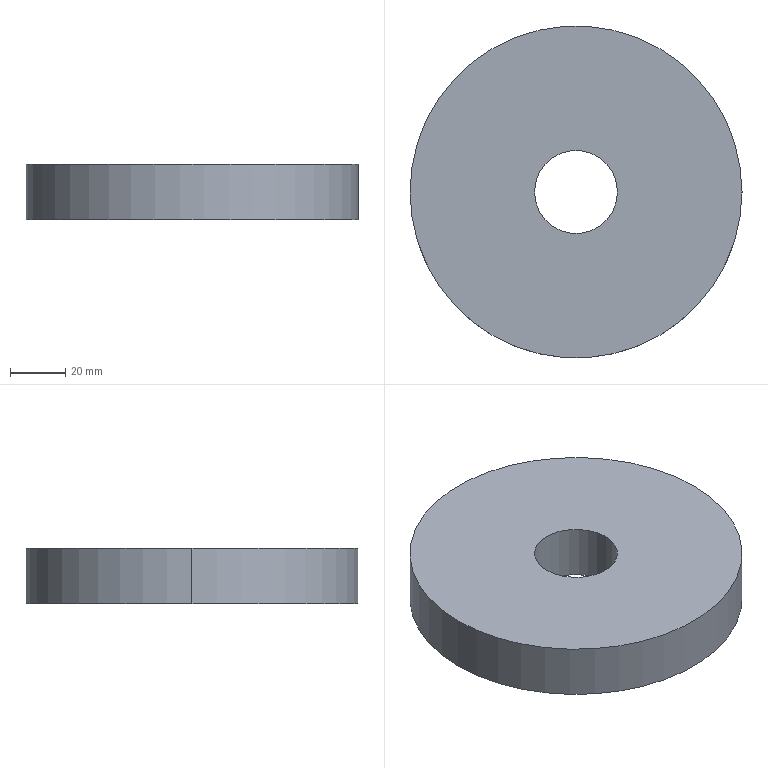Part | SolidWorks | features Extrusion 1 | 1 solid | 6 faces | box 120 x 120 x 20 mm | volume 212058 mm3 | cylinder 4 | plane 2 | commonest cylinder face diameters 30 x2 120 x2
STEP:
#1=CARTESIAN_POINT('',(-15.,0.,10.));
#2=VERTEX_POINT('',#1);
#3=CARTESIAN_POINT('',(15.,0.,10.));
#4=VERTEX_POINT('',#3);
#5=CARTESIAN_POINT('',(0.,0.,10.));
#6=DIRECTION('',(0.,0.,1.));
#7=DIRECTION('',(1.,0.,0.));
#8=AXIS2_PLACEMENT_3D('',#5,#6,#7);
#9=CIRCLE('',#8,15.);
#10=EDGE_CURVE('',#2,#4,#9,.T.);
#11=ORIENTED_EDGE('',*,*,#10,.T.);
#12=CARTESIAN_POINT('',(15.,0.,-10.));
#13=VERTEX_POINT('',#12);
#14=CARTESIAN_POINT('',(15.,0.,10.));
#15=DIRECTION('',(0.,0.,-1.));
#16=VECTOR('',#15,1000.);
#17=LINE('',#14,#16);
#18=EDGE_CURVE('',#4,#13,#17,.T.);
#19=ORIENTED_EDGE('',*,*,#18,.T.);
#20=CARTESIAN_POINT('',(-15.,0.,-10.));
#21=VERTEX_POINT('',#20);
#22=CARTESIAN_POINT('',(0.,0.,-10.));
#23=DIRECTION('',(0.,0.,1.));
#24=DIRECTION('',(1.,0.,0.));
#25=AXIS2_PLACEMENT_3D('',#22,#23,#24);
#26=CIRCLE('',#25,15.);
#27=EDGE_CURVE('',#21,#13,#26,.T.);
#28=ORIENTED_EDGE('',*,*,#27,.F.);
#29=CARTESIAN_POINT('',(-15.,0.,10.));
#30=DIRECTION('',(0.,0.,-1.));
#31=VECTOR('',#30,1000.);
#32=LINE('',#29,#31);
#33=EDGE_CURVE('',#2,#21,#32,.T.);
#34=ORIENTED_EDGE('',*,*,#33,.F.);
#35=EDGE_LOOP('',(#11,#19,#28,#34));
#36=FACE_OUTER_BOUND('',#35,.T.);
#37=CARTESIAN_POINT('',(0.,0.,10.));
#38=DIRECTION('',(0.,0.,-1.));
#39=DIRECTION('',(-1.,0.,0.));
#40=AXIS2_PLACEMENT_3D('',#37,#38,#39);
#41=CYLINDRICAL_SURFACE('',#40,15.);
#42=ADVANCED_FACE('',(#36),#41,.F.);
#43=CARTESIAN_POINT('',(60.,0.,10.));
#44=VERTEX_POINT('',#43);
#45=CARTESIAN_POINT('',(-60.,0.,10.));
#46=VERTEX_POINT('',#45);
#47=CARTESIAN_POINT('',(0.,0.,10.));
#48=DIRECTION('',(0.,0.,1.));
#49=DIRECTION('',(1.,0.,0.));
#50=AXIS2_PLACEMENT_3D('',#47,#48,#49);
#51=CIRCLE('',#50,60.);
#52=EDGE_CURVE('',#44,#46,#51,.T.);
#53=ORIENTED_EDGE('',*,*,#52,.F.);
#54=CARTESIAN_POINT('',(60.,0.,-10.));
#55=VERTEX_POINT('',#54);
#56=CARTESIAN_POINT('',(60.,0.,10.));
#57=DIRECTION('',(0.,0.,-1.));
#58=VECTOR('',#57,1000.);
#59=LINE('',#56,#58);
#60=EDGE_CURVE('',#44,#55,#59,.T.);
#61=ORIENTED_EDGE('',*,*,#60,.T.);
#62=CARTESIAN_POINT('',(-60.,0.,-10.));
#63=VERTEX_POINT('',#62);
#64=CARTESIAN_POINT('',(0.,0.,-10.));
#65=DIRECTION('',(0.,0.,1.));
#66=DIRECTION('',(1.,0.,0.));
#67=AXIS2_PLACEMENT_3D('',#64,#65,#66);
#68=CIRCLE('',#67,60.);
#69=EDGE_CURVE('',#55,#63,#68,.T.);
#70=ORIENTED_EDGE('',*,*,#69,.T.);
#71=CARTESIAN_POINT('',(-60.,0.,10.));
#72=DIRECTION('',(0.,0.,-1.));
#73=VECTOR('',#72,1000.);
#74=LINE('',#71,#73);
#75=EDGE_CURVE('',#46,#63,#74,.T.);
#76=ORIENTED_EDGE('',*,*,#75,.F.);
#77=EDGE_LOOP('',(#53,#61,#70,#76));
#78=FACE_OUTER_BOUND('',#77,.T.);
#79=CARTESIAN_POINT('',(0.,0.,10.));
#80=DIRECTION('',(0.,0.,-1.));
#81=DIRECTION('',(-1.,0.,0.));
#82=AXIS2_PLACEMENT_3D('',#79,#80,#81);
#83=CYLINDRICAL_SURFACE('',#82,60.);
#84=ADVANCED_FACE('',(#78),#83,.T.);
#85=CARTESIAN_POINT('',(0.,0.,10.));
#86=DIRECTION('',(0.,0.,1.));
#87=DIRECTION('',(1.,0.,0.));
#88=AXIS2_PLACEMENT_3D('',#85,#86,#87);
#89=CIRCLE('',#88,60.);
#90=EDGE_CURVE('',#46,#44,#89,.T.);
#91=ORIENTED_EDGE('',*,*,#90,.T.);
#92=ORIENTED_EDGE('',*,*,#52,.T.);
#93=EDGE_LOOP('',(#91,#92));
#94=FACE_OUTER_BOUND('',#93,.T.);
#95=ORIENTED_EDGE('',*,*,#10,.F.);
#96=CARTESIAN_POINT('',(0.,0.,10.));
#97=DIRECTION('',(0.,0.,1.));
#98=DIRECTION('',(1.,0.,0.));
#99=AXIS2_PLACEMENT_3D('',#96,#97,#98);
#100=CIRCLE('',#99,15.);
#101=EDGE_CURVE('',#4,#2,#100,.T.);
#102=ORIENTED_EDGE('',*,*,#101,.F.);
#103=EDGE_LOOP('',(#95,#102));
#104=FACE_BOUND('',#103,.T.);
#105=CARTESIAN_POINT('',(0.,0.,10.));
#106=DIRECTION('',(0.,0.,1.));
#107=DIRECTION('',(1.,0.,0.));
#108=AXIS2_PLACEMENT_3D('',#105,#106,#107);
#109=PLANE('',#108);
#110=ADVANCED_FACE('',(#94,#104),#109,.T.);
#111=CARTESIAN_POINT('',(0.,0.,-10.));
#112=DIRECTION('',(0.,0.,1.));
#113=DIRECTION('',(1.,0.,0.));
#114=AXIS2_PLACEMENT_3D('',#111,#112,#113);
#115=CIRCLE('',#114,60.);
#116=EDGE_CURVE('',#63,#55,#115,.T.);
#117=ORIENTED_EDGE('',*,*,#116,.F.);
#118=ORIENTED_EDGE('',*,*,#69,.F.);
#119=EDGE_LOOP('',(#117,#118));
#120=FACE_OUTER_BOUND('',#119,.T.);
#121=ORIENTED_EDGE('',*,*,#27,.T.);
#122=CARTESIAN_POINT('',(0.,0.,-10.));
#123=DIRECTION('',(0.,0.,1.));
#124=DIRECTION('',(1.,0.,0.));
#125=AXIS2_PLACEMENT_3D('',#122,#123,#124);
#126=CIRCLE('',#125,15.);
#127=EDGE_CURVE('',#13,#21,#126,.T.);
#128=ORIENTED_EDGE('',*,*,#127,.T.);
#129=EDGE_LOOP('',(#121,#128));
#130=FACE_BOUND('',#129,.T.);
#131=CARTESIAN_POINT('',(0.,0.,-10.));
#132=DIRECTION('',(0.,0.,1.));
#133=DIRECTION('',(1.,0.,0.));
#134=AXIS2_PLACEMENT_3D('',#131,#132,#133);
#135=PLANE('',#134);
#136=ADVANCED_FACE('',(#120,#130),#135,.F.);
#137=ORIENTED_EDGE('',*,*,#60,.F.);
#138=ORIENTED_EDGE('',*,*,#90,.F.);
#139=ORIENTED_EDGE('',*,*,#75,.T.);
#140=ORIENTED_EDGE('',*,*,#116,.T.);
#141=EDGE_LOOP('',(#137,#138,#139,#140));
#142=FACE_OUTER_BOUND('',#141,.T.);
#143=CARTESIAN_POINT('',(0.,0.,10.));
#144=DIRECTION('',(0.,0.,-1.));
#145=DIRECTION('',(-1.,0.,0.));
#146=AXIS2_PLACEMENT_3D('',#143,#144,#145);
#147=CYLINDRICAL_SURFACE('',#146,60.);
#148=ADVANCED_FACE('',(#142),#147,.T.);
#149=ORIENTED_EDGE('',*,*,#18,.F.);
#150=ORIENTED_EDGE('',*,*,#101,.T.);
#151=ORIENTED_EDGE('',*,*,#33,.T.);
#152=ORIENTED_EDGE('',*,*,#127,.F.);
#153=EDGE_LOOP('',(#149,#150,#151,#152));
#154=FACE_OUTER_BOUND('',#153,.T.);
#155=CARTESIAN_POINT('',(0.,0.,10.));
#156=DIRECTION('',(0.,0.,-1.));
#157=DIRECTION('',(-1.,0.,0.));
#158=AXIS2_PLACEMENT_3D('',#155,#156,#157);
#159=CYLINDRICAL_SURFACE('',#158,15.);
#160=ADVANCED_FACE('',(#154),#159,.F.);
#161=CLOSED_SHELL('',(#42,#84,#110,#136,#148,#160));
#162=MANIFOLD_SOLID_BREP('',#161);
#163=CARTESIAN_POINT('',(0.,0.,0.));
#164=DIRECTION('',(0.,0.,1.));
#165=DIRECTION('',(1.,0.,0.));
#166=AXIS2_PLACEMENT_3D('',#163,#164,#165);
#167=(LENGTH_UNIT()NAMED_UNIT(*)SI_UNIT(.MILLI.,.METRE.));
#168=UNCERTAINTY_MEASURE_WITH_UNIT(LENGTH_MEASURE(0.00001),#167,'','');
#169=(NAMED_UNIT(*)PLANE_ANGLE_UNIT()SI_UNIT($,.RADIAN.));
#170=(NAMED_UNIT(*)SI_UNIT($,.STERADIAN.)SOLID_ANGLE_UNIT());
#171=(GEOMETRIC_REPRESENTATION_CONTEXT(3)GLOBAL_UNCERTAINTY_ASSIGNED_CONTEXT((#168))GLOBAL_UNIT_ASSIGNED_CONTEXT((#167,#169,#170))REPRESENTATION_CONTEXT('',''));
#172=ADVANCED_BREP_SHAPE_REPRESENTATION('',(#162,#166),#171);